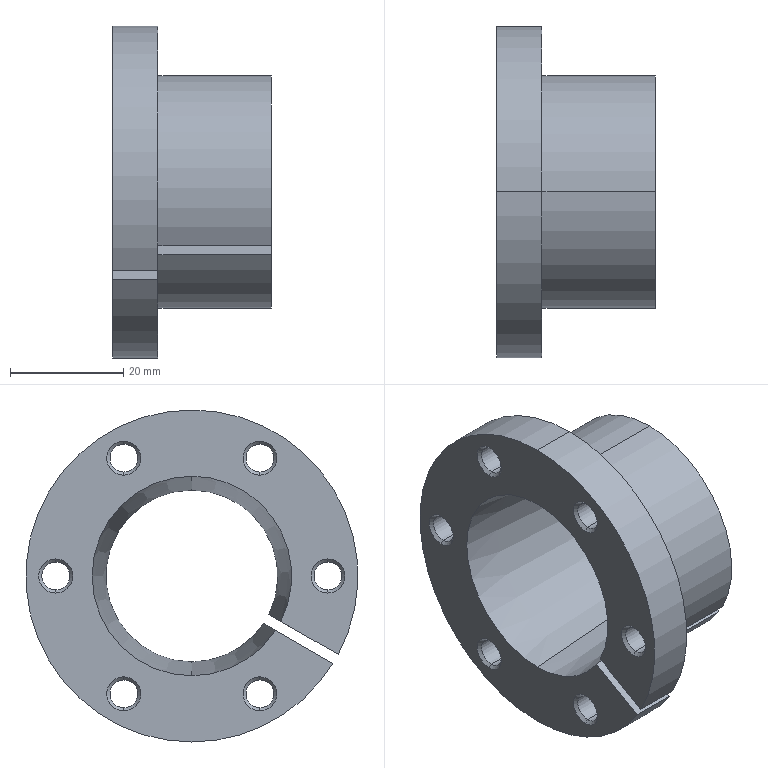Part | STEP file | MLR30body | 1 solid | 50 faces | box 28 x 58.56 x 58.56 mm | volume 23041 mm3 | cone 27 | cylinder 18 | plane 5 | commonest cylinder face diameters 4.917 x12 41 x3 58.56 x3